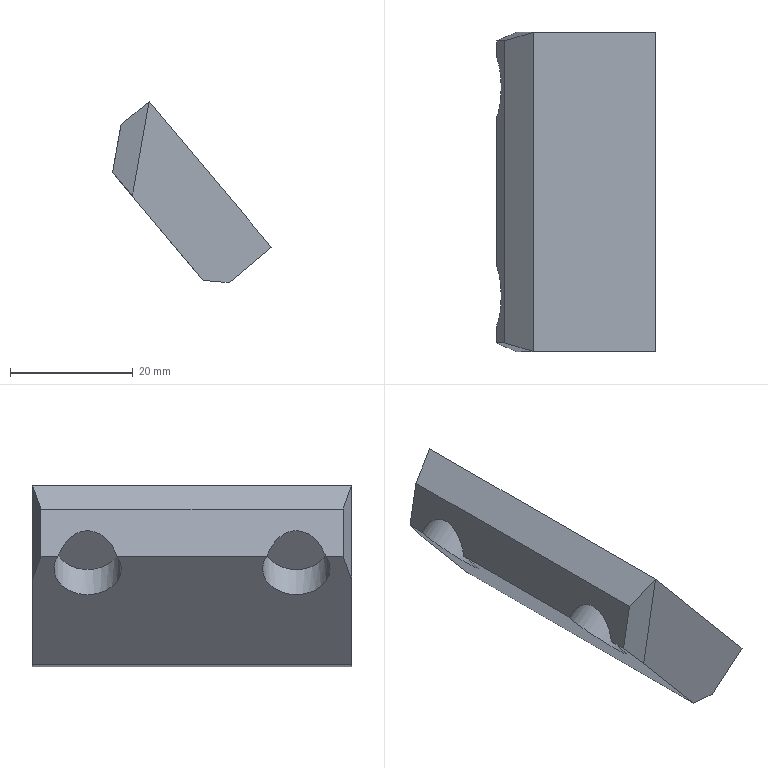Part | NX | features solid 2 | 1 solid | 14 faces | box 25.883 x 52 x 29.532 mm | volume 16989 mm3 | plane 12 | cylinder 2 | commonest cylinder face diameters 11 x2
STEP:
#1=CARTESIAN_POINT('',(1223.237,64.16,14.107));
#2=VERTEX_POINT('',#1);
#3=CARTESIAN_POINT('',(1223.237,73.84,14.107));
#4=VERTEX_POINT('',#3);
#5=CARTESIAN_POINT('',(1224.918,69.,12.103));
#6=DIRECTION('',(0.766,0.,0.6428));
#7=DIRECTION('',(0.6428,0.,-0.766));
#8=AXIS2_PLACEMENT_3D('',#5,#6,#7);
#9=ELLIPSE('',#8,5.507,5.5);
#10=EDGE_CURVE('',#2,#4,#9,.T.);
#11=ORIENTED_EDGE('',*,*,#10,.T.);
#12=CARTESIAN_POINT('',(1223.237,98.16,14.107));
#13=VERTEX_POINT('',#12);
#14=CARTESIAN_POINT('',(1223.237,60.,14.107));
#15=DIRECTION('',(0.,1.,0.));
#16=VECTOR('',#15,1000.);
#17=LINE('',#14,#16);
#18=EDGE_CURVE('',#4,#13,#17,.T.);
#19=ORIENTED_EDGE('',*,*,#18,.T.);
#20=CARTESIAN_POINT('',(1223.237,107.84,14.107));
#21=VERTEX_POINT('',#20);
#22=CARTESIAN_POINT('',(1224.918,103.,12.103));
#23=DIRECTION('',(0.766,0.,0.6428));
#24=DIRECTION('',(0.6428,0.,-0.766));
#25=AXIS2_PLACEMENT_3D('',#22,#23,#24);
#26=ELLIPSE('',#25,5.507,5.5);
#27=EDGE_CURVE('',#21,#13,#26,.F.);
#28=ORIENTED_EDGE('',*,*,#27,.F.);
#29=CARTESIAN_POINT('',(1223.237,110.598,14.107));
#30=VERTEX_POINT('',#29);
#31=CARTESIAN_POINT('',(1223.237,60.,14.107));
#32=DIRECTION('',(0.,1.,0.));
#33=VECTOR('',#32,1000.);
#34=LINE('',#31,#33);
#35=EDGE_CURVE('',#21,#30,#34,.T.);
#36=ORIENTED_EDGE('',*,*,#35,.T.);
#37=CARTESIAN_POINT('',(1226.469,112.,10.255));
#38=VERTEX_POINT('',#37);
#39=CARTESIAN_POINT('',(1214.823,106.948,24.134));
#40=DIRECTION('',(0.6192,0.2686,-0.7379));
#41=VECTOR('',#40,1000.);
#42=LINE('',#39,#41);
#43=EDGE_CURVE('',#30,#38,#42,.T.);
#44=ORIENTED_EDGE('',*,*,#43,.T.);
#45=CARTESIAN_POINT('',(1237.999,112.,-3.486));
#46=VERTEX_POINT('',#45);
#47=CARTESIAN_POINT('',(1223.237,112.,14.107));
#48=DIRECTION('',(0.6428,0.,-0.766));
#49=VECTOR('',#48,1000.);
#50=LINE('',#47,#49);
#51=EDGE_CURVE('',#38,#46,#50,.T.);
#52=ORIENTED_EDGE('',*,*,#51,.T.);
#53=CARTESIAN_POINT('',(1237.999,60.,-3.486));
#54=VERTEX_POINT('',#53);
#55=CARTESIAN_POINT('',(1237.999,60.,-3.486));
#56=DIRECTION('',(0.,1.,0.));
#57=VECTOR('',#56,1000.);
#58=LINE('',#55,#57);
#59=EDGE_CURVE('',#54,#46,#58,.T.);
#60=ORIENTED_EDGE('',*,*,#59,.F.);
#61=CARTESIAN_POINT('',(1226.469,60.,10.255));
#62=VERTEX_POINT('',#61);
#63=CARTESIAN_POINT('',(1223.237,60.,14.107));
#64=DIRECTION('',(0.6428,0.,-0.766));
#65=VECTOR('',#64,1000.);
#66=LINE('',#63,#65);
#67=EDGE_CURVE('',#62,#54,#66,.T.);
#68=ORIENTED_EDGE('',*,*,#67,.F.);
#69=CARTESIAN_POINT('',(1223.237,61.402,14.107));
#70=VERTEX_POINT('',#69);
#71=CARTESIAN_POINT('',(1223.47,61.301,13.829));
#72=DIRECTION('',(0.6192,-0.2686,-0.7379));
#73=VECTOR('',#72,1000.);
#74=LINE('',#71,#73);
#75=EDGE_CURVE('',#70,#62,#74,.T.);
#76=ORIENTED_EDGE('',*,*,#75,.F.);
#77=CARTESIAN_POINT('',(1223.237,60.,14.107));
#78=DIRECTION('',(0.,1.,0.));
#79=VECTOR('',#78,1000.);
#80=LINE('',#77,#79);
#81=EDGE_CURVE('',#70,#2,#80,.T.);
#82=ORIENTED_EDGE('',*,*,#81,.T.);
#83=EDGE_LOOP('',(#11,#19,#28,#36,#44,#52,#60,#68,#76,#82));
#84=FACE_BOUND('',#83,.T.);
#85=CARTESIAN_POINT('',(1223.237,60.,14.107));
#86=DIRECTION('',(-0.766,0.,-0.6428));
#87=DIRECTION('',(-0.6428,0.,0.766));
#88=AXIS2_PLACEMENT_3D('',#85,#86,#87);
#89=PLANE('',#88);
#90=ADVANCED_FACE('',(#84),#89,.T.);
#91=CARTESIAN_POINT('',(1229.194,112.,25.677));
#92=VERTEX_POINT('',#91);
#93=CARTESIAN_POINT('',(1249.12,112.,1.929));
#94=VERTEX_POINT('',#93);
#95=CARTESIAN_POINT('',(1229.194,112.,25.677));
#96=DIRECTION('',(0.6428,0.,-0.766));
#97=VECTOR('',#96,1000.);
#98=LINE('',#95,#97);
#99=EDGE_CURVE('',#92,#94,#98,.T.);
#100=ORIENTED_EDGE('',*,*,#99,.F.);
#101=CARTESIAN_POINT('',(1229.194,60.,25.677));
#102=VERTEX_POINT('',#101);
#103=CARTESIAN_POINT('',(1229.194,60.,25.677));
#104=DIRECTION('',(0.,1.,0.));
#105=VECTOR('',#104,1000.);
#106=LINE('',#103,#105);
#107=EDGE_CURVE('',#102,#92,#106,.T.);
#108=ORIENTED_EDGE('',*,*,#107,.F.);
#109=CARTESIAN_POINT('',(1249.12,60.,1.929));
#110=VERTEX_POINT('',#109);
#111=CARTESIAN_POINT('',(1229.194,60.,25.677));
#112=DIRECTION('',(0.6428,0.,-0.766));
#113=VECTOR('',#112,1000.);
#114=LINE('',#111,#113);
#115=EDGE_CURVE('',#102,#110,#114,.T.);
#116=ORIENTED_EDGE('',*,*,#115,.T.);
#117=CARTESIAN_POINT('',(1249.12,60.,1.929));
#118=DIRECTION('',(0.,1.,0.));
#119=VECTOR('',#118,1000.);
#120=LINE('',#117,#119);
#121=EDGE_CURVE('',#110,#94,#120,.T.);
#122=ORIENTED_EDGE('',*,*,#121,.T.);
#123=EDGE_LOOP('',(#100,#108,#116,#122));
#124=FACE_BOUND('',#123,.T.);
#125=CARTESIAN_POINT('',(1229.194,112.,25.677));
#126=DIRECTION('',(0.766,0.,0.6428));
#127=DIRECTION('',(0.6428,0.,-0.766));
#128=AXIS2_PLACEMENT_3D('',#125,#126,#127);
#129=PLANE('',#128);
#130=ADVANCED_FACE('',(#124),#129,.T.);
#131=ORIENTED_EDGE('',*,*,#81,.F.);
#132=CARTESIAN_POINT('',(1224.597,61.402,21.82));
#133=VERTEX_POINT('',#132);
#134=CARTESIAN_POINT('',(1223.237,61.402,14.107));
#135=DIRECTION('',(0.1736,0.,0.9848));
#136=VECTOR('',#135,1000.);
#137=LINE('',#134,#136);
#138=EDGE_CURVE('',#70,#133,#137,.T.);
#139=ORIENTED_EDGE('',*,*,#138,.T.);
#140=CARTESIAN_POINT('',(1224.597,110.598,21.82));
#141=VERTEX_POINT('',#140);
#142=CARTESIAN_POINT('',(1224.597,60.,21.82));
#143=DIRECTION('',(0.,1.,0.));
#144=VECTOR('',#143,1000.);
#145=LINE('',#142,#144);
#146=EDGE_CURVE('',#133,#141,#145,.T.);
#147=ORIENTED_EDGE('',*,*,#146,.T.);
#148=CARTESIAN_POINT('',(1223.237,110.598,14.107));
#149=DIRECTION('',(0.1736,0.,0.9848));
#150=VECTOR('',#149,1000.);
#151=LINE('',#148,#150);
#152=EDGE_CURVE('',#30,#141,#151,.T.);
#153=ORIENTED_EDGE('',*,*,#152,.F.);
#154=ORIENTED_EDGE('',*,*,#35,.F.);
#155=CARTESIAN_POINT('',(1222.571,103.,10.325));
#156=DIRECTION('',(-0.9848,0.,0.1736));
#157=DIRECTION('',(0.1736,0.,0.9848));
#158=AXIS2_PLACEMENT_3D('',#155,#156,#157);
#159=ELLIPSE('',#158,8.085,5.5);
#160=EDGE_CURVE('',#21,#13,#159,.F.);
#161=ORIENTED_EDGE('',*,*,#160,.T.);
#162=ORIENTED_EDGE('',*,*,#18,.F.);
#163=CARTESIAN_POINT('',(1222.571,69.,10.325));
#164=DIRECTION('',(-0.9848,0.,0.1736));
#165=DIRECTION('',(0.1736,0.,0.9848));
#166=AXIS2_PLACEMENT_3D('',#163,#164,#165);
#167=ELLIPSE('',#166,8.085,5.5);
#168=EDGE_CURVE('',#2,#4,#167,.T.);
#169=ORIENTED_EDGE('',*,*,#168,.F.);
#170=EDGE_LOOP('',(#131,#139,#147,#153,#154,#161,#162,#169));
#171=FACE_BOUND('',#170,.T.);
#172=CARTESIAN_POINT('',(1223.237,60.,14.107));
#173=DIRECTION('',(0.9848,0.,-0.1736));
#174=DIRECTION('',(-0.1736,0.,-0.9848));
#175=AXIS2_PLACEMENT_3D('',#172,#173,#174);
#176=PLANE('',#175);
#177=ADVANCED_FACE('',(#171),#176,.F.);
#178=CARTESIAN_POINT('',(1242.226,112.,-3.856));
#179=VERTEX_POINT('',#178);
#180=CARTESIAN_POINT('',(1237.999,112.,-3.486));
#181=DIRECTION('',(0.9962,0.,-0.08716));
#182=VECTOR('',#181,1000.);
#183=LINE('',#180,#182);
#184=EDGE_CURVE('',#46,#179,#183,.T.);
#185=ORIENTED_EDGE('',*,*,#184,.T.);
#186=CARTESIAN_POINT('',(1242.226,60.,-3.856));
#187=VERTEX_POINT('',#186);
#188=CARTESIAN_POINT('',(1242.226,60.,-3.856));
#189=DIRECTION('',(0.,1.,0.));
#190=VECTOR('',#189,1000.);
#191=LINE('',#188,#190);
#192=EDGE_CURVE('',#187,#179,#191,.T.);
#193=ORIENTED_EDGE('',*,*,#192,.F.);
#194=CARTESIAN_POINT('',(1237.999,60.,-3.486));
#195=DIRECTION('',(0.9962,0.,-0.08716));
#196=VECTOR('',#195,1000.);
#197=LINE('',#194,#196);
#198=EDGE_CURVE('',#54,#187,#197,.T.);
#199=ORIENTED_EDGE('',*,*,#198,.F.);
#200=ORIENTED_EDGE('',*,*,#59,.T.);
#201=EDGE_LOOP('',(#185,#193,#199,#200));
#202=FACE_BOUND('',#201,.T.);
#203=CARTESIAN_POINT('',(1237.999,60.,-3.486));
#204=DIRECTION('',(-0.08716,0.,-0.9962));
#205=DIRECTION('',(-0.9962,0.,0.08716));
#206=AXIS2_PLACEMENT_3D('',#203,#204,#205);
#207=PLANE('',#206);
#208=ADVANCED_FACE('',(#202),#207,.T.);
#209=CARTESIAN_POINT('',(1229.188,60.,25.672));
#210=VERTEX_POINT('',#209);
#211=CARTESIAN_POINT('',(1224.836,61.329,22.02));
#212=DIRECTION('',(0.7459,-0.2278,0.6259));
#213=VECTOR('',#212,1000.);
#214=LINE('',#211,#213);
#215=EDGE_CURVE('',#133,#210,#214,.T.);
#216=ORIENTED_EDGE('',*,*,#215,.F.);
#217=ORIENTED_EDGE('',*,*,#138,.F.);
#218=ORIENTED_EDGE('',*,*,#75,.T.);
#219=CARTESIAN_POINT('',(1239.966,60.,86.799));
#220=DIRECTION('',(-0.1736,0.,-0.9848));
#221=VECTOR('',#220,1000.);
#222=LINE('',#219,#221);
#223=EDGE_CURVE('',#210,#62,#222,.T.);
#224=ORIENTED_EDGE('',*,*,#223,.F.);
#225=EDGE_LOOP('',(#216,#217,#218,#224));
#226=FACE_BOUND('',#225,.T.);
#227=CARTESIAN_POINT('',(1219.514,69.099,114.776));
#228=DIRECTION('',(-0.3368,-0.9397,0.05939));
#229=DIRECTION('',(-0.9254,0.342,0.1632));
#230=AXIS2_PLACEMENT_3D('',#227,#228,#229);
#231=PLANE('',#230);
#232=ADVANCED_FACE('',(#226),#231,.T.);
#233=ORIENTED_EDGE('',*,*,#152,.T.);
#234=CARTESIAN_POINT('',(1229.188,112.,25.672));
#235=VERTEX_POINT('',#234);
#236=CARTESIAN_POINT('',(1216.,107.972,14.606));
#237=DIRECTION('',(0.7459,0.2278,0.6259));
#238=VECTOR('',#237,1000.);
#239=LINE('',#236,#238);
#240=EDGE_CURVE('',#141,#235,#239,.T.);
#241=ORIENTED_EDGE('',*,*,#240,.T.);
#242=CARTESIAN_POINT('',(1239.966,112.,86.799));
#243=DIRECTION('',(0.1736,0.,0.9848));
#244=VECTOR('',#243,1000.);
#245=LINE('',#242,#244);
#246=EDGE_CURVE('',#38,#235,#245,.T.);
#247=ORIENTED_EDGE('',*,*,#246,.F.);
#248=ORIENTED_EDGE('',*,*,#43,.F.);
#249=EDGE_LOOP('',(#233,#241,#247,#248));
#250=FACE_BOUND('',#249,.T.);
#251=CARTESIAN_POINT('',(1219.514,102.901,114.776));
#252=DIRECTION('',(0.3368,-0.9397,-0.05939));
#253=DIRECTION('',(-0.9254,-0.342,0.1632));
#254=AXIS2_PLACEMENT_3D('',#251,#252,#253);
#255=PLANE('',#254);
#256=ADVANCED_FACE('',(#250),#255,.F.);
#257=CARTESIAN_POINT('',(1242.226,112.,-3.856));
#258=DIRECTION('',(0.766,0.,0.6428));
#259=VECTOR('',#258,1000.);
#260=LINE('',#257,#259);
#261=EDGE_CURVE('',#179,#94,#260,.T.);
#262=ORIENTED_EDGE('',*,*,#261,.T.);
#263=ORIENTED_EDGE('',*,*,#121,.F.);
#264=CARTESIAN_POINT('',(1242.226,60.,-3.856));
#265=DIRECTION('',(0.766,0.,0.6428));
#266=VECTOR('',#265,1000.);
#267=LINE('',#264,#266);
#268=EDGE_CURVE('',#187,#110,#267,.T.);
#269=ORIENTED_EDGE('',*,*,#268,.F.);
#270=ORIENTED_EDGE('',*,*,#192,.T.);
#271=EDGE_LOOP('',(#262,#263,#269,#270));
#272=FACE_BOUND('',#271,.T.);
#273=CARTESIAN_POINT('',(1242.226,60.,-3.856));
#274=DIRECTION('',(0.6428,0.,-0.766));
#275=DIRECTION('',(-0.766,0.,-0.6428));
#276=AXIS2_PLACEMENT_3D('',#273,#274,#275);
#277=PLANE('',#276);
#278=ADVANCED_FACE('',(#272),#277,.T.);
#279=ORIENTED_EDGE('',*,*,#146,.F.);
#280=ORIENTED_EDGE('',*,*,#215,.T.);
#281=CARTESIAN_POINT('',(1224.597,60.,21.82));
#282=DIRECTION('',(0.766,0.,0.6428));
#283=VECTOR('',#282,1000.);
#284=LINE('',#281,#283);
#285=EDGE_CURVE('',#210,#102,#284,.T.);
#286=ORIENTED_EDGE('',*,*,#285,.T.);
#287=ORIENTED_EDGE('',*,*,#107,.T.);
#288=CARTESIAN_POINT('',(1224.597,112.,21.82));
#289=DIRECTION('',(0.766,0.,0.6428));
#290=VECTOR('',#289,1000.);
#291=LINE('',#288,#290);
#292=EDGE_CURVE('',#235,#92,#291,.T.);
#293=ORIENTED_EDGE('',*,*,#292,.F.);
#294=ORIENTED_EDGE('',*,*,#240,.F.);
#295=EDGE_LOOP('',(#279,#280,#286,#287,#293,#294));
#296=FACE_BOUND('',#295,.T.);
#297=CARTESIAN_POINT('',(1224.597,60.,21.82));
#298=DIRECTION('',(0.6428,0.,-0.766));
#299=DIRECTION('',(-0.766,0.,-0.6428));
#300=AXIS2_PLACEMENT_3D('',#297,#298,#299);
#301=PLANE('',#300);
#302=ADVANCED_FACE('',(#296),#301,.F.);
#303=ORIENTED_EDGE('',*,*,#261,.F.);
#304=ORIENTED_EDGE('',*,*,#184,.F.);
#305=ORIENTED_EDGE('',*,*,#51,.F.);
#306=ORIENTED_EDGE('',*,*,#246,.T.);
#307=ORIENTED_EDGE('',*,*,#292,.T.);
#308=ORIENTED_EDGE('',*,*,#99,.T.);
#309=EDGE_LOOP('',(#303,#304,#305,#306,#307,#308));
#310=FACE_BOUND('',#309,.T.);
#311=CARTESIAN_POINT('',(1222.141,112.,89.942));
#312=DIRECTION('',(0.,1.,0.));
#313=DIRECTION('',(-0.1736,0.,-0.9848));
#314=AXIS2_PLACEMENT_3D('',#311,#312,#313);
#315=PLANE('',#314);
#316=ADVANCED_FACE('',(#310),#315,.T.);
#317=ORIENTED_EDGE('',*,*,#115,.F.);
#318=ORIENTED_EDGE('',*,*,#285,.F.);
#319=ORIENTED_EDGE('',*,*,#223,.T.);
#320=ORIENTED_EDGE('',*,*,#67,.T.);
#321=ORIENTED_EDGE('',*,*,#198,.T.);
#322=ORIENTED_EDGE('',*,*,#268,.T.);
#323=EDGE_LOOP('',(#317,#318,#319,#320,#321,#322));
#324=FACE_BOUND('',#323,.T.);
#325=CARTESIAN_POINT('',(1222.141,60.,89.942));
#326=DIRECTION('',(0.,1.,0.));
#327=DIRECTION('',(-0.1736,0.,-0.9848));
#328=AXIS2_PLACEMENT_3D('',#325,#326,#327);
#329=PLANE('',#328);
#330=ADVANCED_FACE('',(#324),#329,.F.);
#331=ORIENTED_EDGE('',*,*,#160,.F.);
#332=ORIENTED_EDGE('',*,*,#27,.T.);
#333=EDGE_LOOP('',(#331,#332));
#334=FACE_BOUND('',#333,.T.);
#335=CARTESIAN_POINT('',(1227.185,103.,20.719));
#336=VERTEX_POINT('',#335);
#337=CARTESIAN_POINT('',(1230.506,103.,16.334));
#338=DIRECTION('',(0.7972,0.,0.6037));
#339=DIRECTION('',(-0.6037,0.,0.7972));
#340=AXIS2_PLACEMENT_3D('',#337,#338,#339);
#341=CIRCLE('',#340,5.5);
#342=EDGE_CURVE('',#336,#336,#341,.T.);
#343=ORIENTED_EDGE('',*,*,#342,.T.);
#344=EDGE_LOOP('',(#343));
#345=FACE_BOUND('',#344,.T.);
#346=CARTESIAN_POINT('',(1222.534,103.,10.297));
#347=DIRECTION('',(0.7972,0.,0.6037));
#348=DIRECTION('',(0.6037,0.,-0.7972));
#349=AXIS2_PLACEMENT_3D('',#346,#347,#348);
#350=CYLINDRICAL_SURFACE('',#349,5.5);
#351=ADVANCED_FACE('',(#334,#345),#350,.F.);
#352=ORIENTED_EDGE('',*,*,#342,.F.);
#353=EDGE_LOOP('',(#352));
#354=FACE_BOUND('',#353,.T.);
#355=CARTESIAN_POINT('',(1230.506,103.,16.334));
#356=DIRECTION('',(-0.7972,0.,-0.6037));
#357=DIRECTION('',(-0.6037,0.,0.7972));
#358=AXIS2_PLACEMENT_3D('',#355,#356,#357);
#359=PLANE('',#358);
#360=ADVANCED_FACE('',(#354),#359,.T.);
#361=ORIENTED_EDGE('',*,*,#10,.F.);
#362=ORIENTED_EDGE('',*,*,#168,.T.);
#363=EDGE_LOOP('',(#361,#362));
#364=FACE_BOUND('',#363,.T.);
#365=CARTESIAN_POINT('',(1233.826,69.,11.95));
#366=VERTEX_POINT('',#365);
#367=CARTESIAN_POINT('',(1230.506,69.,16.334));
#368=DIRECTION('',(-0.7972,0.,-0.6037));
#369=DIRECTION('',(0.6037,0.,-0.7972));
#370=AXIS2_PLACEMENT_3D('',#367,#368,#369);
#371=CIRCLE('',#370,5.5);
#372=EDGE_CURVE('',#366,#366,#371,.T.);
#373=ORIENTED_EDGE('',*,*,#372,.F.);
#374=EDGE_LOOP('',(#373));
#375=FACE_BOUND('',#374,.T.);
#376=CARTESIAN_POINT('',(1222.534,69.,10.297));
#377=DIRECTION('',(0.7972,0.,0.6037));
#378=DIRECTION('',(0.6037,0.,-0.7972));
#379=AXIS2_PLACEMENT_3D('',#376,#377,#378);
#380=CYLINDRICAL_SURFACE('',#379,5.5);
#381=ADVANCED_FACE('',(#364,#375),#380,.F.);
#382=ORIENTED_EDGE('',*,*,#372,.T.);
#383=EDGE_LOOP('',(#382));
#384=FACE_BOUND('',#383,.T.);
#385=CARTESIAN_POINT('',(1230.506,69.,16.334));
#386=DIRECTION('',(0.7972,0.,0.6037));
#387=DIRECTION('',(0.6037,0.,-0.7972));
#388=AXIS2_PLACEMENT_3D('',#385,#386,#387);
#389=PLANE('',#388);
#390=ADVANCED_FACE('',(#384),#389,.F.);
#391=CLOSED_SHELL('',(#90,#130,#177,#208,#232,#256,#278,#302,#316,#330,#351,#360,#381,#390));
#392=MANIFOLD_SOLID_BREP('',#391);
#393=(LENGTH_UNIT()NAMED_UNIT(*)SI_UNIT(.MILLI.,.METRE.));
#394=UNCERTAINTY_MEASURE_WITH_UNIT(LENGTH_MEASURE(0.00001),#393,'','');
#395=(NAMED_UNIT(*)PLANE_ANGLE_UNIT()SI_UNIT($,.RADIAN.));
#396=(NAMED_UNIT(*)SI_UNIT($,.STERADIAN.)SOLID_ANGLE_UNIT());
#397=(GEOMETRIC_REPRESENTATION_CONTEXT(3)GLOBAL_UNCERTAINTY_ASSIGNED_CONTEXT((#394))GLOBAL_UNIT_ASSIGNED_CONTEXT((#393,#395,#396))REPRESENTATION_CONTEXT('',''));
#398=ADVANCED_BREP_SHAPE_REPRESENTATION('',(#392),#397);